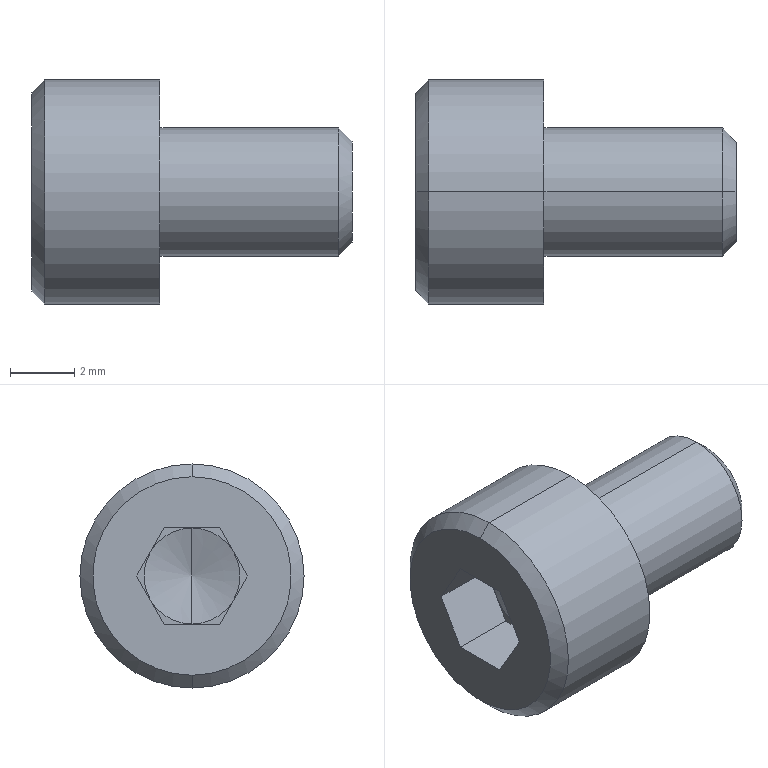Part | STEP file | 0243_318_SCB4-6 | 1 solid | 25 faces | box 10 x 7 x 7 mm | volume 210.032 mm3 | plane 15 | cone 6 | cylinder 4 | commonest cylinder face diameters 4 x2 7 x2